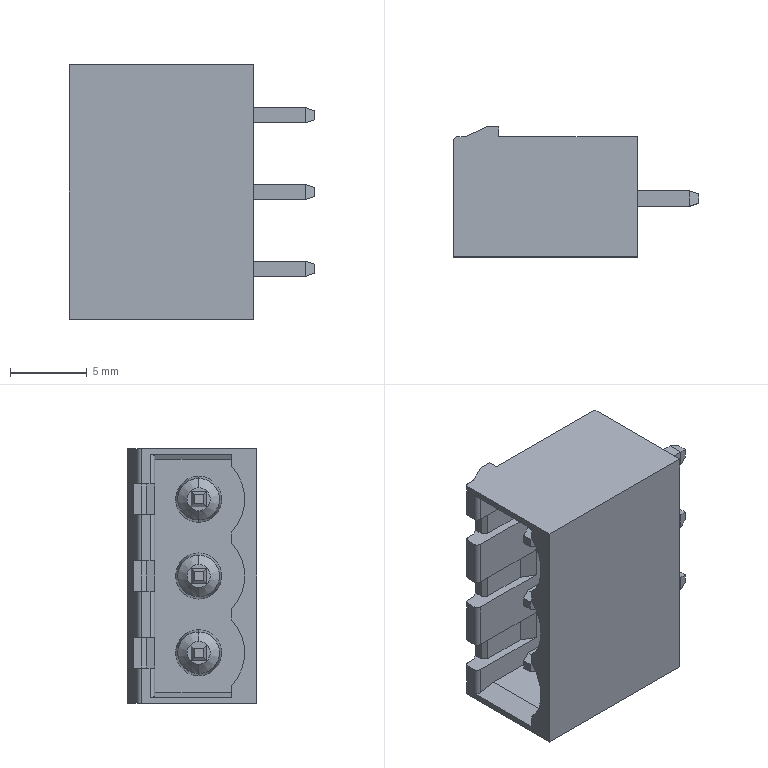Part | SolidWorks | features BaseBody 1 | 1 solid | 123 faces | box 16 x 8.47 x 16.6 mm | volume 886.614 mm3 | plane 100 | cone 12 | cylinder 11 | commonest cylinder face diameters 0.6 x8 6.12 x3